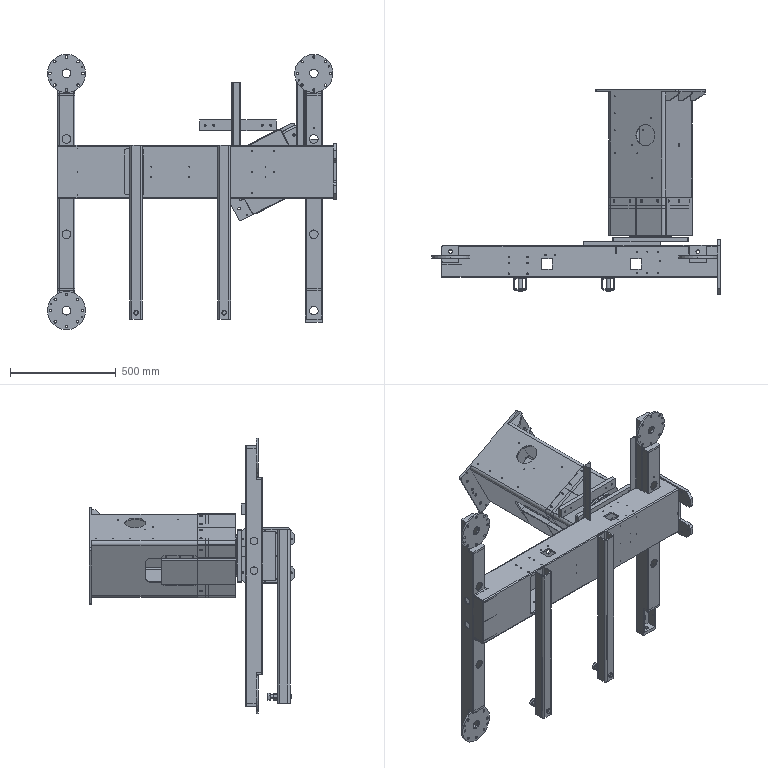Part | SolidWorks | features CompositeCurve 17, InContextFeatHolder 10 | 43 solids | 2359 faces | box 1365 x 969.6 x 1300 mm | volume 30670521 mm3 | cylinder 1264 | plane 658 | cone 407 | torus 26 | spline 4 | commonest cylinder face diameters 4.2 x118 5 x102 8.5 x92 10 x80 12 x76 6.8 x68